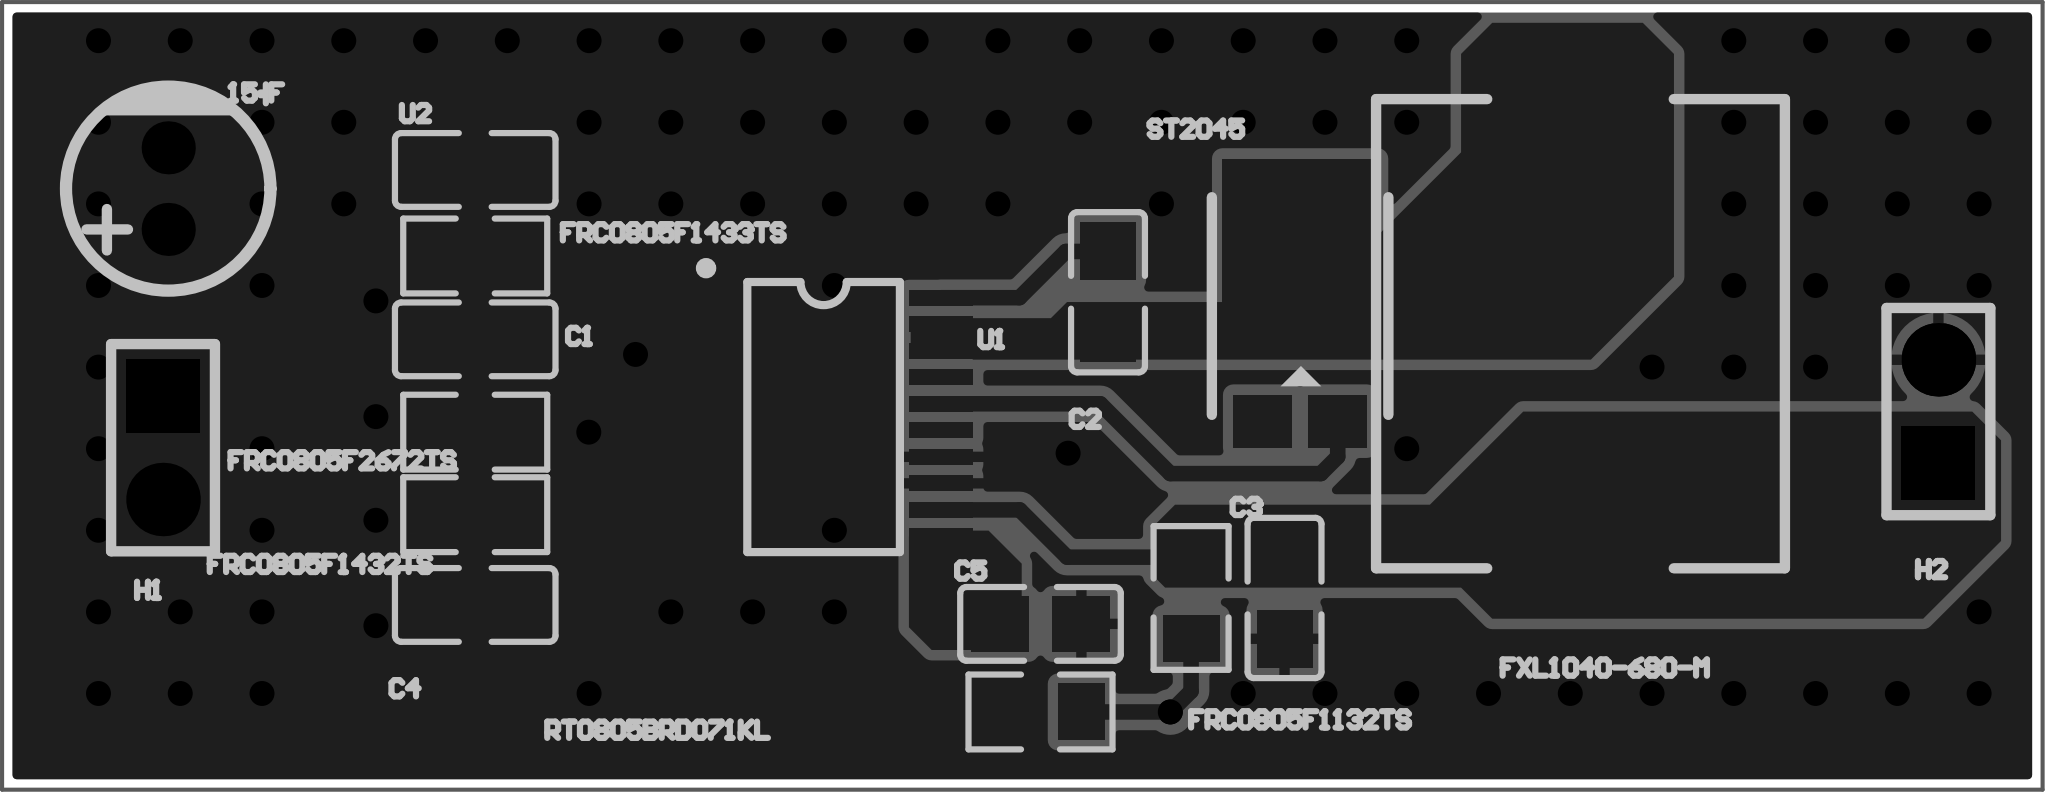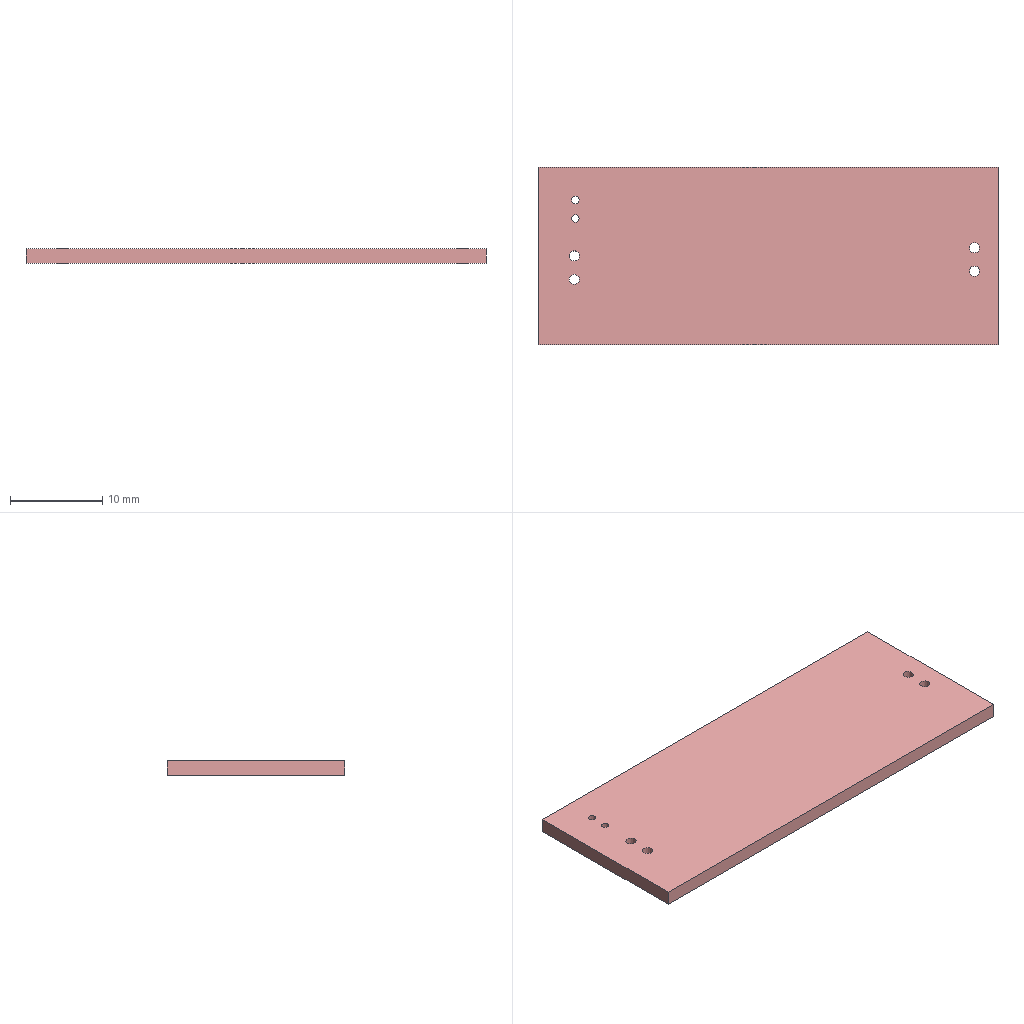Circuit board layout | Altium Designer | box 49.9 x 19.3 x 1.6 mm
Layer stack:
# Altium Designer layer stack of  (unit mm; dielectric type: 0 none, 1 core, 2 prepreg, 3 surface material)
index,name,kind,layer,copper_thickness_mm,dielectric_type,dielectric_thickness_mm,dielectric_material,dielectric_constant
0,Top Paste Mask Layer,other,,,,,,
1,Top Silkscreen Layer,other,,,,,,
2,Top Solder Mask Layer,dielectric,,,3,0.01,,3.3
3,Top Layer,copper,Top Layer,0.035,,,,
4,Dielectric1,dielectric,,,3,1.51,FR4,4.5
5,Bottom Layer,copper,Bottom Layer,0.035,,,,
6,Bottom Solder Mask Layer,dielectric,,,3,0.01,,3.3
7,Bottom Silkscreen Layer,other,,,,,,
8,Bottom Paste Mask Layer,other,,,,,,
# drill layer pairs: low layer,high layer
drill_pair,Top Layer,Bottom Layer
Part placement:
Designator,Comment,Layer,Footprint,Center-X(mm),Center-Y(mm),Rotation
15µF,LKMB1102A150MF,TopLayer,CAP-TH_BD5.0-P2.00-D0.8-FD,82.169,93.726,90
C1,CL21A106KAYNNNE,TopLayer,C0805,89.678,90.032,180
C2,CL21A106KAYNNNE,TopLayer,C0805,105.156,91.186,90
C3,CL21A106KAYNNNE,TopLayer,C0805,109.474,83.693,270
C4,FCC0805B681K500DT,TopLayer,C0805,89.678,83.522,180
C5,FM21X273K101ECG,TopLayer,C0805,103.505,83.058,0
FRC0805F1132TS,,TopLayer,R0805,107.188,83.693,270
FRC0805F1432TS,,TopLayer,R0805,89.678,85.734,180
FRC0805F1433TS,,TopLayer,R0805,89.678,92.075,180
FRC0805F2672TS,,TopLayer,R0805,89.678,87.757,0
FXL1040-680-M,68µH,TopLayer,IND-SMD_L11.5-W10.0_104CDMCCDS,116.713,90.17,270
RT0805BRD071KL,,TopLayer,R0805,103.505,80.899,180
ST2045,ST2045,TopLayer,TO-277_3P-L5.4-W4.0-LS6.5-BR,109.855,90.043,270
U1,LM5576MHX/NOPB,TopLayer,HTSSOP-20_L6.5-W4.4-P0.65-LS6.4-BL-EP3.0,98.199,88.127,270
U2,CL21B104KCFNNNE,TopLayer,C0805,89.678,94.183,180
H1,,TopLayer,HDR-TH_2P-P2.54-V-M-1,82.042,87.376,270
H2,,TopLayer,HDR-TH_2P-P2.54-V-M-1,125.468,88.261,90
Pad and via stacks:
# Altium Designer via and pad stacks of  (unit mm). Each distinct definition once, with the count of objects using it.
# via: kind,start_layer,end_layer,hole_mm,diameter_mm,mode(0 simple;1 top-mid-bottom;2 full stack),diameter_per_layer,count,example_net
# pad: kind,layer,hole_mm,hole_type(0 round;1 square;2 slot),plating,top_size,top_shape(1 round;2 rect;3 octagon;9 rounded rect),mid_size,bottom_size,mode,footprint,size_per_layer,count,example
pad,Multi-Layer,0.8,0,plated,1.3x1.3,1,1.3x1.3,1.3x1.3,0,CAP-TH_BD5.0-P2.00-D0.8-FD,,2,15\u03BCF.1
pad,Multi-Layer,1.1,0,plated,1.8x1.8,1,1.8x1.8,1.8x1.8,0,HDR-TH_2P-P2.54-V-M-1,,2,H1.2
pad,Multi-Layer,1.1,0,plated,1.8x1.8,2,1.8x1.8,1.8x1.8,0,HDR-TH_2P-P2.54-V-M-1,,2,H1.1
pad,Top Layer,0,0,plated,1.41x1.35,2,1.41x1.35,1.41x1.35,0,C0805,,12,C1.2
pad,Top Layer,0,0,plated,1.133x1.377,2,1.133x1.377,1.133x1.377,0,R0805,,10,FRC0805F1132TS.2
pad,Top Layer,0,0,plated,3.5x4.1,2,3.5x4.1,3.5x4.1,0,IND-SMD_L11.5-W10.0_104CDMCCDS,,2,FXL1040-680-M.1
pad,Top Layer,0,0,plated,3.8x4.8,2,3.8x4.8,3.8x4.8,0,TO-277_3P-L5.4-W4.0-LS6.5-BR,,1,ST2045.2
pad,Top Layer,0,0,plated,1.29x1.422,2,1.29x1.422,1.29x1.422,0,TO-277_3P-L5.4-W4.0-LS6.5-BR,,2,ST2045.1
pad,Top Layer,0,0,plated,2.4x3,2,2.4x3,2.4x3,0,HTSSOP-20_L6.5-W4.4-P0.65-LS6.4-BL-EP3.0,,1,U1.21
pad,Top Layer,0,0,plated,0.3683x1.562,2,0.3683x1.562,0.3683x1.562,0,HTSSOP-20_L6.5-W4.4-P0.65-LS6.4-BL-EP3.0,,20,U1.11
via,Top Layer,Bottom Layer,0.3048,0.61,0,,99,$2N16
Copper pours:
name,layer,net,type(0 solid;1 hatched;2 none)
Top Layer-GND,Top Layer,GND,0
Bottom Layer-GND,Bottom Layer,GND,0